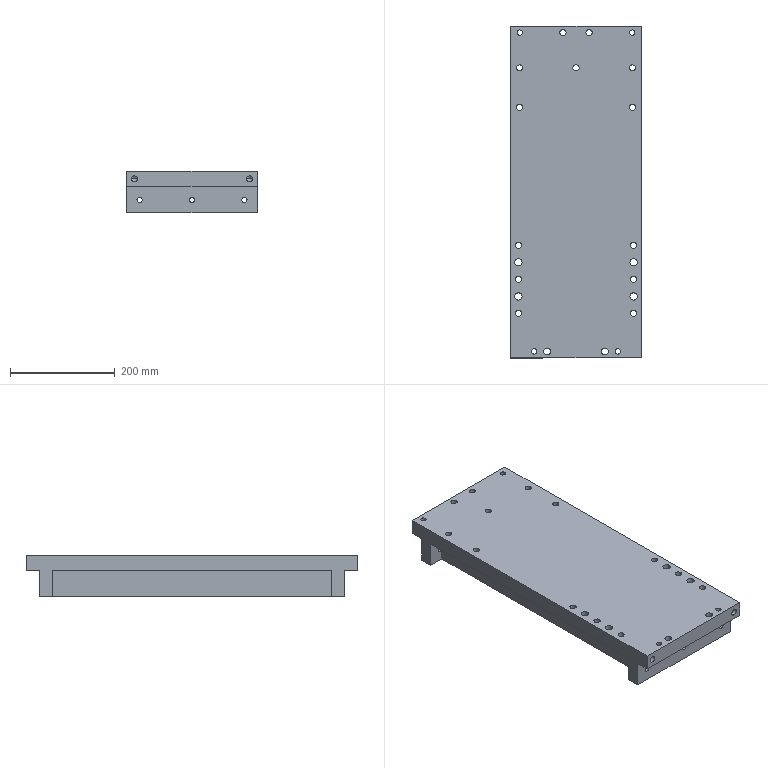Part | STEP file | MAT BAN CO LOGO | 1 solid | 101 faces | box 250 x 633.6 x 80 mm | volume 6070480 mm3 | cylinder 66 | plane 27 | cone 8 | commonest cylinder face diameters 11.835 x34 10.106 x20 14 x8 13 x4